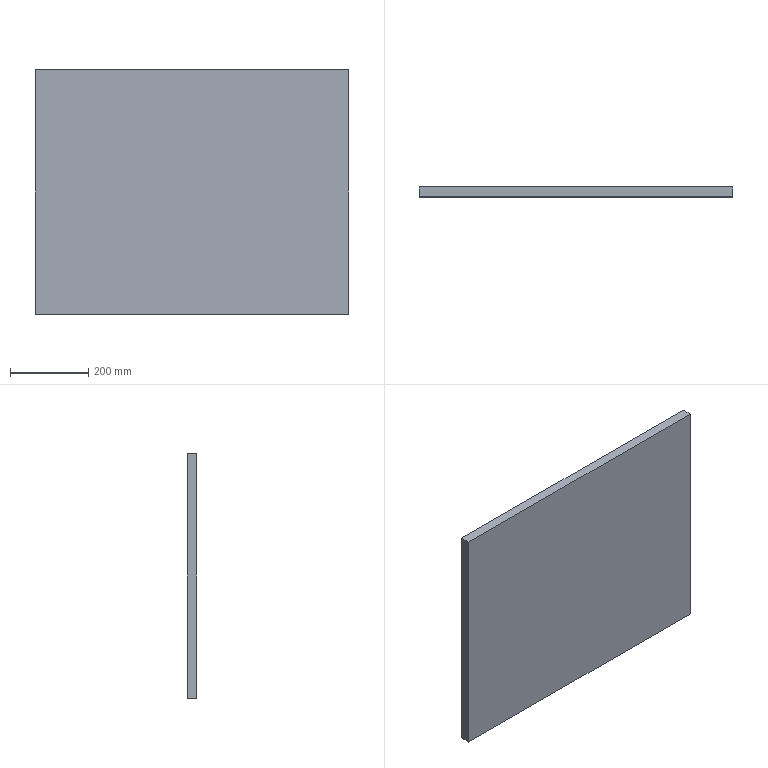Part | SolidWorks | features SplitBody 1 | 1 solid | 6 faces | box 800 x 25 x 624 mm | volume 12480000 mm3 | plane 6
STEP:
#1=CARTESIAN_POINT('',(4331.,918.44,600.));
#2=VERTEX_POINT('',#1);
#3=CARTESIAN_POINT('',(4331.,918.44,1224.));
#4=VERTEX_POINT('',#3);
#5=CARTESIAN_POINT('',(4331.,918.44,600.));
#6=DIRECTION('',(0.,0.,1.));
#7=VECTOR('',#6,1000.);
#8=LINE('',#5,#7);
#9=EDGE_CURVE('',#2,#4,#8,.T.);
#10=ORIENTED_EDGE('',*,*,#9,.T.);
#11=CARTESIAN_POINT('',(3531.,918.44,1224.));
#12=VERTEX_POINT('',#11);
#13=CARTESIAN_POINT('',(3531.,918.44,1224.));
#14=DIRECTION('',(-1.,0.,0.));
#15=VECTOR('',#14,1000.);
#16=LINE('',#13,#15);
#17=EDGE_CURVE('',#4,#12,#16,.T.);
#18=ORIENTED_EDGE('',*,*,#17,.T.);
#19=CARTESIAN_POINT('',(3531.,918.44,600.));
#20=VERTEX_POINT('',#19);
#21=CARTESIAN_POINT('',(3531.,918.44,600.));
#22=DIRECTION('',(0.,0.,-1.));
#23=VECTOR('',#22,1000.);
#24=LINE('',#21,#23);
#25=EDGE_CURVE('',#12,#20,#24,.T.);
#26=ORIENTED_EDGE('',*,*,#25,.T.);
#27=CARTESIAN_POINT('',(3531.,918.44,600.));
#28=DIRECTION('',(1.,0.,0.));
#29=VECTOR('',#28,1000.);
#30=LINE('',#27,#29);
#31=EDGE_CURVE('',#20,#2,#30,.T.);
#32=ORIENTED_EDGE('',*,*,#31,.T.);
#33=EDGE_LOOP('',(#10,#18,#26,#32));
#34=FACE_OUTER_BOUND('',#33,.T.);
#35=CARTESIAN_POINT('',(3531.,918.44,600.));
#36=DIRECTION('',(0.,-1.,0.));
#37=DIRECTION('',(1.,0.,0.));
#38=AXIS2_PLACEMENT_3D('',#35,#36,#37);
#39=PLANE('',#38);
#40=ADVANCED_FACE('',(#34),#39,.T.);
#41=CARTESIAN_POINT('',(3531.,943.44,1224.));
#42=VERTEX_POINT('',#41);
#43=CARTESIAN_POINT('',(3531.,918.44,1224.));
#44=DIRECTION('',(0.,1.,0.));
#45=VECTOR('',#44,1000.);
#46=LINE('',#43,#45);
#47=EDGE_CURVE('',#12,#42,#46,.T.);
#48=ORIENTED_EDGE('',*,*,#47,.F.);
#49=ORIENTED_EDGE('',*,*,#17,.F.);
#50=CARTESIAN_POINT('',(4331.,943.44,1224.));
#51=VERTEX_POINT('',#50);
#52=CARTESIAN_POINT('',(4331.,918.44,1224.));
#53=DIRECTION('',(0.,-1.,0.));
#54=VECTOR('',#53,1000.);
#55=LINE('',#52,#54);
#56=EDGE_CURVE('',#51,#4,#55,.T.);
#57=ORIENTED_EDGE('',*,*,#56,.F.);
#58=CARTESIAN_POINT('',(3531.,943.44,1224.));
#59=DIRECTION('',(1.,0.,0.));
#60=VECTOR('',#59,1000.);
#61=LINE('',#58,#60);
#62=EDGE_CURVE('',#42,#51,#61,.T.);
#63=ORIENTED_EDGE('',*,*,#62,.F.);
#64=EDGE_LOOP('',(#48,#49,#57,#63));
#65=FACE_OUTER_BOUND('',#64,.T.);
#66=CARTESIAN_POINT('',(3531.,918.44,1224.));
#67=DIRECTION('',(0.,0.,-1.));
#68=DIRECTION('',(0.,1.,0.));
#69=AXIS2_PLACEMENT_3D('',#66,#67,#68);
#70=PLANE('',#69);
#71=ADVANCED_FACE('',(#65),#70,.F.);
#72=ORIENTED_EDGE('',*,*,#56,.T.);
#73=ORIENTED_EDGE('',*,*,#9,.F.);
#74=CARTESIAN_POINT('',(4331.,943.44,600.));
#75=VERTEX_POINT('',#74);
#76=CARTESIAN_POINT('',(4331.,918.44,600.));
#77=DIRECTION('',(0.,-1.,0.));
#78=VECTOR('',#77,1000.);
#79=LINE('',#76,#78);
#80=EDGE_CURVE('',#75,#2,#79,.T.);
#81=ORIENTED_EDGE('',*,*,#80,.F.);
#82=CARTESIAN_POINT('',(4331.,943.44,1224.));
#83=DIRECTION('',(0.,0.,-1.));
#84=VECTOR('',#83,1000.);
#85=LINE('',#82,#84);
#86=EDGE_CURVE('',#51,#75,#85,.T.);
#87=ORIENTED_EDGE('',*,*,#86,.F.);
#88=EDGE_LOOP('',(#72,#73,#81,#87));
#89=FACE_OUTER_BOUND('',#88,.T.);
#90=CARTESIAN_POINT('',(4331.,918.44,1224.));
#91=DIRECTION('',(-1.,0.,0.));
#92=DIRECTION('',(0.,0.,-1.));
#93=AXIS2_PLACEMENT_3D('',#90,#91,#92);
#94=PLANE('',#93);
#95=ADVANCED_FACE('',(#89),#94,.F.);
#96=ORIENTED_EDGE('',*,*,#80,.T.);
#97=ORIENTED_EDGE('',*,*,#31,.F.);
#98=CARTESIAN_POINT('',(3531.,943.44,600.));
#99=VERTEX_POINT('',#98);
#100=CARTESIAN_POINT('',(3531.,918.44,600.));
#101=DIRECTION('',(0.,-1.,0.));
#102=VECTOR('',#101,1000.);
#103=LINE('',#100,#102);
#104=EDGE_CURVE('',#99,#20,#103,.T.);
#105=ORIENTED_EDGE('',*,*,#104,.F.);
#106=CARTESIAN_POINT('',(3531.,943.44,600.));
#107=DIRECTION('',(-1.,0.,0.));
#108=VECTOR('',#107,1000.);
#109=LINE('',#106,#108);
#110=EDGE_CURVE('',#75,#99,#109,.T.);
#111=ORIENTED_EDGE('',*,*,#110,.F.);
#112=EDGE_LOOP('',(#96,#97,#105,#111));
#113=FACE_OUTER_BOUND('',#112,.T.);
#114=CARTESIAN_POINT('',(3531.,918.44,600.));
#115=DIRECTION('',(0.,0.,1.));
#116=DIRECTION('',(0.,-1.,0.));
#117=AXIS2_PLACEMENT_3D('',#114,#115,#116);
#118=PLANE('',#117);
#119=ADVANCED_FACE('',(#113),#118,.F.);
#120=ORIENTED_EDGE('',*,*,#104,.T.);
#121=ORIENTED_EDGE('',*,*,#25,.F.);
#122=ORIENTED_EDGE('',*,*,#47,.T.);
#123=CARTESIAN_POINT('',(3531.,943.44,1224.));
#124=DIRECTION('',(0.,0.,1.));
#125=VECTOR('',#124,1000.);
#126=LINE('',#123,#125);
#127=EDGE_CURVE('',#99,#42,#126,.T.);
#128=ORIENTED_EDGE('',*,*,#127,.F.);
#129=EDGE_LOOP('',(#120,#121,#122,#128));
#130=FACE_OUTER_BOUND('',#129,.T.);
#131=CARTESIAN_POINT('',(3531.,918.44,1224.));
#132=DIRECTION('',(1.,0.,0.));
#133=DIRECTION('',(0.,0.,1.));
#134=AXIS2_PLACEMENT_3D('',#131,#132,#133);
#135=PLANE('',#134);
#136=ADVANCED_FACE('',(#130),#135,.F.);
#137=ORIENTED_EDGE('',*,*,#62,.T.);
#138=ORIENTED_EDGE('',*,*,#86,.T.);
#139=ORIENTED_EDGE('',*,*,#110,.T.);
#140=ORIENTED_EDGE('',*,*,#127,.T.);
#141=EDGE_LOOP('',(#137,#138,#139,#140));
#142=FACE_OUTER_BOUND('',#141,.T.);
#143=CARTESIAN_POINT('',(3531.,943.44,600.));
#144=DIRECTION('',(0.,-1.,0.));
#145=DIRECTION('',(1.,0.,0.));
#146=AXIS2_PLACEMENT_3D('',#143,#144,#145);
#147=PLANE('',#146);
#148=ADVANCED_FACE('',(#142),#147,.F.);
#149=CLOSED_SHELL('',(#40,#71,#95,#119,#136,#148));
#150=MANIFOLD_SOLID_BREP('',#149);
#151=CARTESIAN_POINT('',(0.,0.,0.));
#152=DIRECTION('',(0.,0.,1.));
#153=DIRECTION('',(1.,0.,0.));
#154=AXIS2_PLACEMENT_3D('',#151,#152,#153);
#155=(LENGTH_UNIT()NAMED_UNIT(*)SI_UNIT(.MILLI.,.METRE.));
#156=UNCERTAINTY_MEASURE_WITH_UNIT(LENGTH_MEASURE(0.00001),#155,'','');
#157=(NAMED_UNIT(*)PLANE_ANGLE_UNIT()SI_UNIT($,.RADIAN.));
#158=(NAMED_UNIT(*)SI_UNIT($,.STERADIAN.)SOLID_ANGLE_UNIT());
#159=(GEOMETRIC_REPRESENTATION_CONTEXT(3)GLOBAL_UNCERTAINTY_ASSIGNED_CONTEXT((#156))GLOBAL_UNIT_ASSIGNED_CONTEXT((#155,#157,#158))REPRESENTATION_CONTEXT('',''));
#160=ADVANCED_BREP_SHAPE_REPRESENTATION('',(#150,#154),#159);